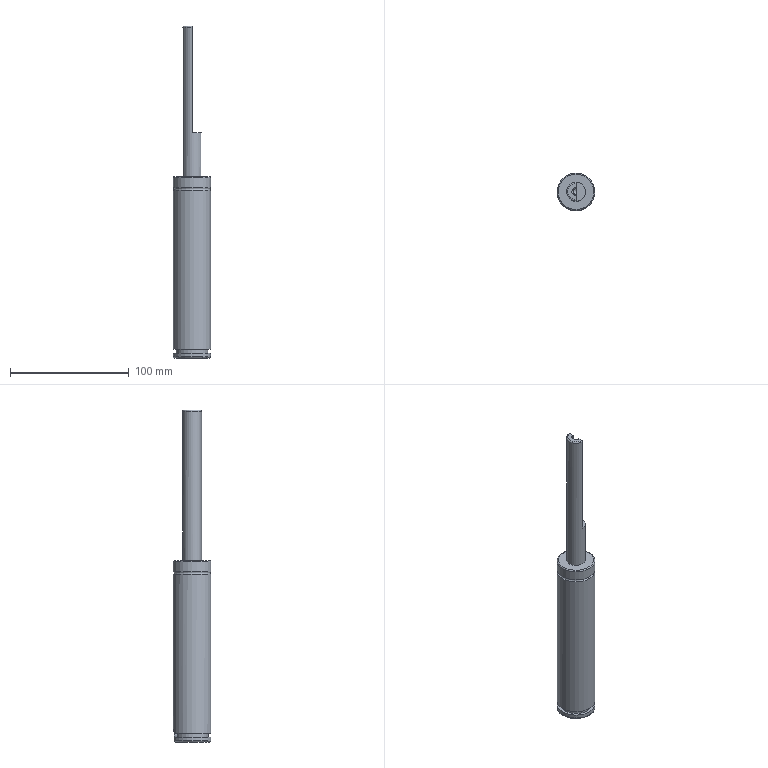Part | NX | features 24 2 | 1 solid | 173 faces | box 31.9 x 31.9 x 280 mm | volume 137246 mm3 | plane 135 | spline 20 | cylinder 10 | cone 4 | torus 4 | commonest cylinder face diameters 4.9 x3 31.9 x3 9.5 x1 11 x1 16 x1 27 x1